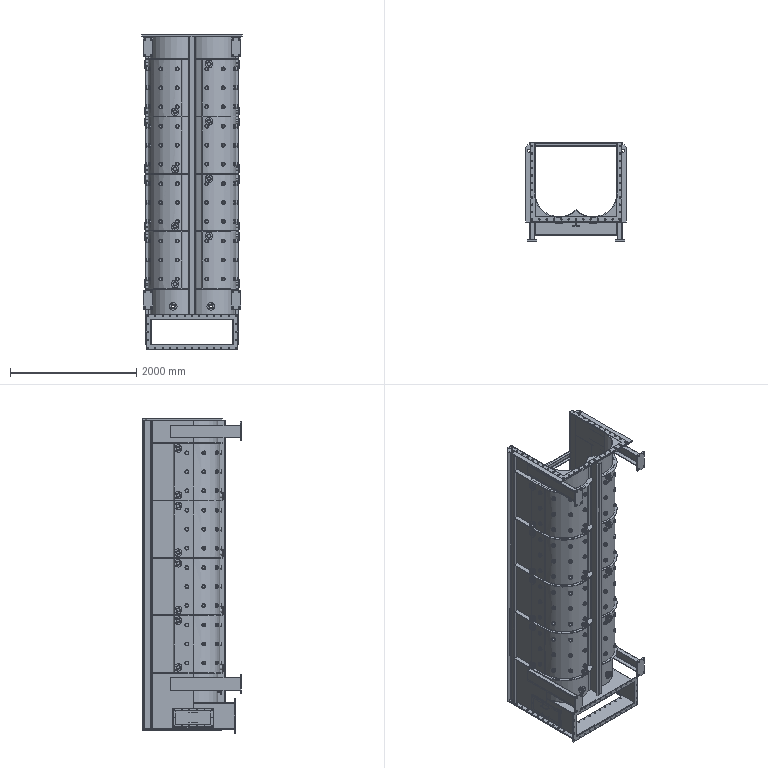Part | SolidWorks | features ReferencePattern 19, LocalLPattern 6, MirrorCompFeat 3, AEMSimFeature 1 | 193 solids | 2556 faces | box 1600 x 1565 x 4990 mm | volume 308843646 mm3 | cylinder 1710 | plane 814 | torus 16 | spline 16 | commonest cylinder face diameters 60 x492 48 x280 14 x208 19.5 x132 24 x128 8.5 x84